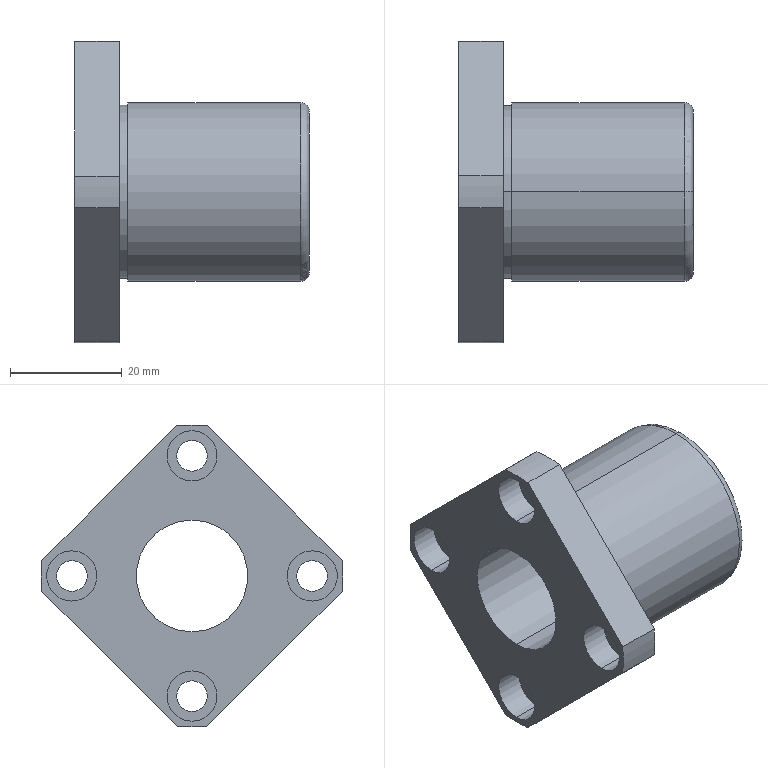Part | STEP file | _LHFSM20.stp | 1 solid | 41 faces | box 42 x 54 x 54 mm | volume 26319 mm3 | cylinder 27 | plane 12 | torus 2 | commonest cylinder face diameters 5.5 x8 9 x8 54 x5 20 x2 31 x2 32 x2